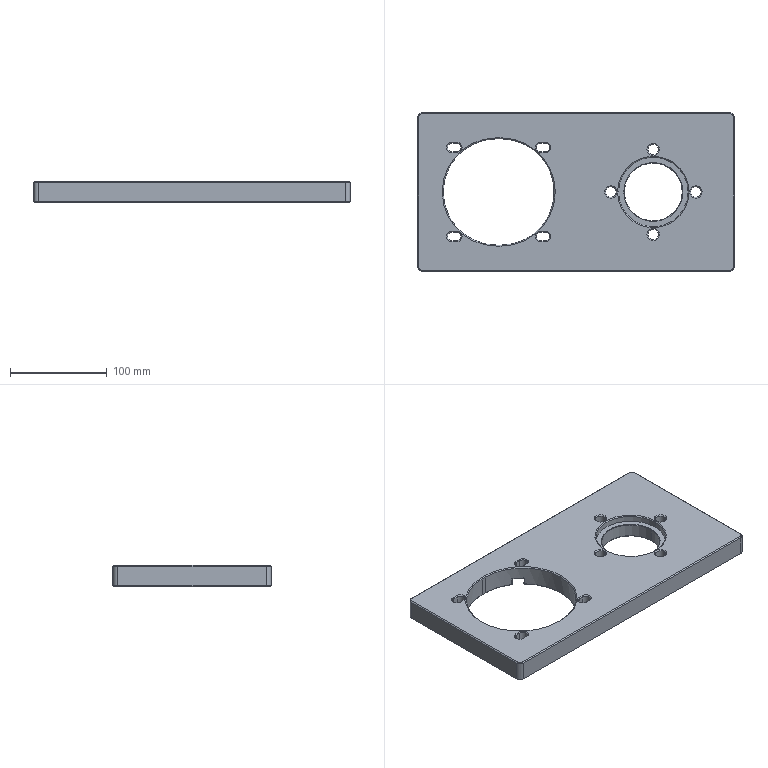NC program | NX | posted with a generic post | part box 328 x 164 x 22 mm
Lines 1 to 31 of 5416:
N10 G17 G21 G94 G90
(DRILLING_COPY_1 , TOOL : ZXZ)
N12 T01 M6
N14 G54
N16 G17 G0 G90 X156.5 Y-74.5 S5000 M3
N18 G43 Z30. H1
N20 G94 G81 G98 Z-1. F250. R3.
N22 Y74.5
N24 X-156.5
N26 Y-74.5
N28 G80
N30 G0 X-156.5 Y-74.5 Z30.
N32 M5
(DRILLING_COPY_COPY_1_COPY , TOOL : 3.3ZT)
N34 T13 M6
N36 G54
N38 G17 G0 G90 X156.5 Y-74.5 S2000 M3
N40 G43 Z30. H13
N42 G94 G83 G98 Z-14.491 F120. Q2. R3.
N44 Y74.5
N46 X-156.5
N48 Y-74.5
N50 G80
N52 G0 X-156.5 Y-74.5 Z30.
N54 M5